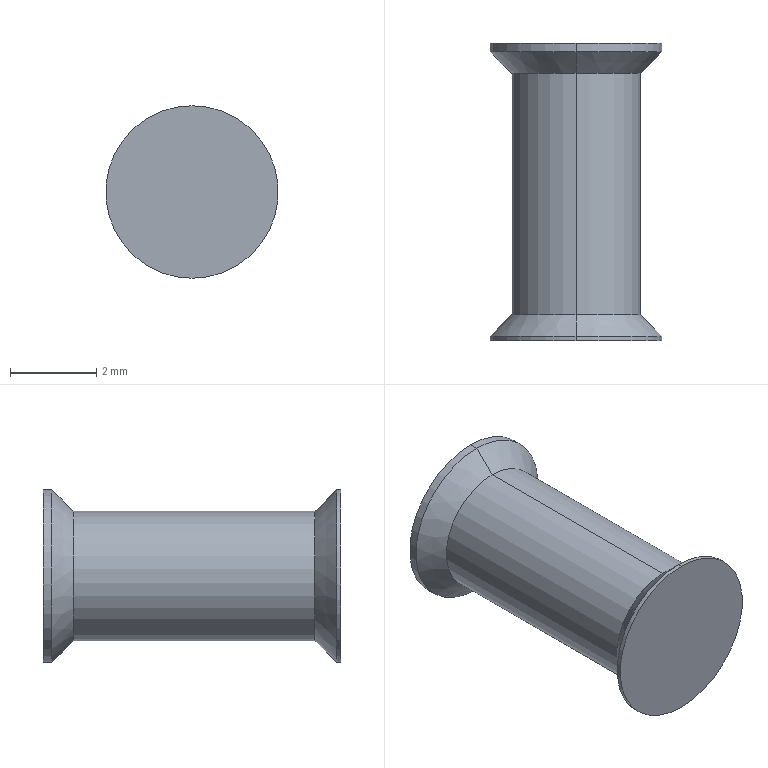Part | SolidWorks | features BaseBody 1 | 1 solid | 18 faces | box 4 x 6.9 x 4 mm | volume 46.627 mm3 | cylinder 8 | cone 6 | torus 2 | plane 2 | commonest cylinder face diameters 4 x4 2 x2 3 x2
STEP:
#1=CARTESIAN_POINT('',(0.,8.1,-1.3));
#2=VERTEX_POINT('',#1);
#3=CARTESIAN_POINT('',(0.,8.1,1.3));
#4=VERTEX_POINT('',#3);
#5=CARTESIAN_POINT('',(0.,8.1,0.));
#6=DIRECTION('',(0.,-1.,0.));
#7=DIRECTION('',(0.,0.,1.));
#8=AXIS2_PLACEMENT_3D('',#5,#6,#7);
#9=CIRCLE('',#8,1.3);
#10=EDGE_CURVE('',#2,#4,#9,.T.);
#11=ORIENTED_EDGE('',*,*,#10,.F.);
#12=CARTESIAN_POINT('',(0.,7.8,-1.));
#13=VERTEX_POINT('',#12);
#14=CARTESIAN_POINT('',(0.,7.8,-1.3));
#15=DIRECTION('',(1.,0.,0.));
#16=DIRECTION('',(0.,0.,-1.));
#17=AXIS2_PLACEMENT_3D('',#14,#15,#16);
#18=CIRCLE('',#17,0.3);
#19=EDGE_CURVE('',#2,#13,#18,.T.);
#20=ORIENTED_EDGE('',*,*,#19,.T.);
#21=CARTESIAN_POINT('',(0.,7.8,1.));
#22=VERTEX_POINT('',#21);
#23=CARTESIAN_POINT('',(0.,7.8,0.));
#24=DIRECTION('',(0.,1.,0.));
#25=DIRECTION('',(0.,0.,1.));
#26=AXIS2_PLACEMENT_3D('',#23,#24,#25);
#27=CIRCLE('',#26,1.);
#28=EDGE_CURVE('',#22,#13,#27,.T.);
#29=ORIENTED_EDGE('',*,*,#28,.F.);
#30=CARTESIAN_POINT('',(0.,7.8,1.3));
#31=DIRECTION('',(-1.,0.,0.));
#32=DIRECTION('',(0.,0.,1.));
#33=AXIS2_PLACEMENT_3D('',#30,#31,#32);
#34=CIRCLE('',#33,0.3);
#35=EDGE_CURVE('',#4,#22,#34,.T.);
#36=ORIENTED_EDGE('',*,*,#35,.F.);
#37=EDGE_LOOP('',(#11,#20,#29,#36));
#38=FACE_OUTER_BOUND('',#37,.T.);
#39=CARTESIAN_POINT('',(0.,7.8,0.));
#40=DIRECTION('',(0.,1.,0.));
#41=DIRECTION('',(0.,0.,1.));
#42=AXIS2_PLACEMENT_3D('',#39,#40,#41);
#43=TOROIDAL_SURFACE('',#42,1.3,0.3);
#44=ADVANCED_FACE('',(#38),#43,.T.);
#45=CARTESIAN_POINT('',(0.,7.8,0.));
#46=DIRECTION('',(0.,1.,0.));
#47=DIRECTION('',(0.,0.,1.));
#48=AXIS2_PLACEMENT_3D('',#45,#46,#47);
#49=CIRCLE('',#48,1.);
#50=EDGE_CURVE('',#13,#22,#49,.T.);
#51=ORIENTED_EDGE('',*,*,#50,.T.);
#52=CARTESIAN_POINT('',(0.,6.3,1.));
#53=VERTEX_POINT('',#52);
#54=CARTESIAN_POINT('',(0.,-2.993,1.));
#55=DIRECTION('',(0.,-1.,0.));
#56=VECTOR('',#55,1000.);
#57=LINE('',#54,#56);
#58=EDGE_CURVE('',#22,#53,#57,.T.);
#59=ORIENTED_EDGE('',*,*,#58,.T.);
#60=CARTESIAN_POINT('',(0.,6.3,-1.));
#61=VERTEX_POINT('',#60);
#62=CARTESIAN_POINT('',(0.,6.3,0.));
#63=DIRECTION('',(0.,-1.,0.));
#64=DIRECTION('',(0.,0.,-1.));
#65=AXIS2_PLACEMENT_3D('',#62,#63,#64);
#66=CIRCLE('',#65,1.);
#67=EDGE_CURVE('',#53,#61,#66,.T.);
#68=ORIENTED_EDGE('',*,*,#67,.T.);
#69=CARTESIAN_POINT('',(0.,-2.993,-1.));
#70=DIRECTION('',(0.,-1.,0.));
#71=VECTOR('',#70,1000.);
#72=LINE('',#69,#71);
#73=EDGE_CURVE('',#13,#61,#72,.T.);
#74=ORIENTED_EDGE('',*,*,#73,.F.);
#75=EDGE_LOOP('',(#51,#59,#68,#74));
#76=FACE_OUTER_BOUND('',#75,.T.);
#77=CARTESIAN_POINT('',(0.,-2.993,0.));
#78=DIRECTION('',(0.,-1.,0.));
#79=DIRECTION('',(0.,0.,-1.));
#80=AXIS2_PLACEMENT_3D('',#77,#78,#79);
#81=CYLINDRICAL_SURFACE('',#80,1.);
#82=ADVANCED_FACE('',(#76),#81,.F.);
#83=CARTESIAN_POINT('',(0.,5.699,0.));
#84=VERTEX_POINT('',#83);
#85=CARTESIAN_POINT('',(0.,6.3,1.));
#86=DIRECTION('',(0.,0.515,0.8572));
#87=VECTOR('',#86,1000.);
#88=LINE('',#85,#87);
#89=EDGE_CURVE('',#84,#53,#88,.T.);
#90=ORIENTED_EDGE('',*,*,#89,.F.);
#91=CARTESIAN_POINT('',(0.,6.3,-1.));
#92=DIRECTION('',(0.,0.515,-0.8572));
#93=VECTOR('',#92,1000.);
#94=LINE('',#91,#93);
#95=EDGE_CURVE('',#84,#61,#94,.T.);
#96=ORIENTED_EDGE('',*,*,#95,.T.);
#97=ORIENTED_EDGE('',*,*,#67,.F.);
#98=EDGE_LOOP('',(#90,#96,#97));
#99=FACE_OUTER_BOUND('',#98,.T.);
#100=CARTESIAN_POINT('',(0.,6.3,0.));
#101=DIRECTION('',(0.,1.,0.));
#102=DIRECTION('',(0.,0.,1.));
#103=AXIS2_PLACEMENT_3D('',#100,#101,#102);
#104=CONICAL_SURFACE('',#103,1.,1.03);
#105=ADVANCED_FACE('',(#99),#104,.F.);
#106=CARTESIAN_POINT('',(0.,7.4,1.5));
#107=VERTEX_POINT('',#106);
#108=CARTESIAN_POINT('',(0.,7.4,-1.5));
#109=VERTEX_POINT('',#108);
#110=CARTESIAN_POINT('',(0.,7.4,0.));
#111=DIRECTION('',(0.,1.,0.));
#112=DIRECTION('',(0.,0.,-1.));
#113=AXIS2_PLACEMENT_3D('',#110,#111,#112);
#114=CIRCLE('',#113,1.5);
#115=EDGE_CURVE('',#107,#109,#114,.T.);
#116=ORIENTED_EDGE('',*,*,#115,.T.);
#117=CARTESIAN_POINT('',(0.,7.9,-2.));
#118=VERTEX_POINT('',#117);
#119=CARTESIAN_POINT('',(0.,7.4,-1.5));
#120=DIRECTION('',(0.,0.7071,-0.7071));
#121=VECTOR('',#120,1000.);
#122=LINE('',#119,#121);
#123=EDGE_CURVE('',#109,#118,#122,.T.);
#124=ORIENTED_EDGE('',*,*,#123,.T.);
#125=CARTESIAN_POINT('',(0.,7.9,2.));
#126=VERTEX_POINT('',#125);
#127=CARTESIAN_POINT('',(0.,7.9,0.));
#128=DIRECTION('',(0.,1.,0.));
#129=DIRECTION('',(0.,0.,-1.));
#130=AXIS2_PLACEMENT_3D('',#127,#128,#129);
#131=CIRCLE('',#130,2.);
#132=EDGE_CURVE('',#126,#118,#131,.T.);
#133=ORIENTED_EDGE('',*,*,#132,.F.);
#134=CARTESIAN_POINT('',(0.,7.4,1.5));
#135=DIRECTION('',(0.,0.7071,0.7071));
#136=VECTOR('',#135,1000.);
#137=LINE('',#134,#136);
#138=EDGE_CURVE('',#107,#126,#137,.T.);
#139=ORIENTED_EDGE('',*,*,#138,.F.);
#140=EDGE_LOOP('',(#116,#124,#133,#139));
#141=FACE_OUTER_BOUND('',#140,.T.);
#142=CARTESIAN_POINT('',(0.,7.4,0.));
#143=DIRECTION('',(0.,1.,0.));
#144=DIRECTION('',(0.,0.,1.));
#145=AXIS2_PLACEMENT_3D('',#142,#143,#144);
#146=CONICAL_SURFACE('',#145,1.5,0.7854);
#147=ADVANCED_FACE('',(#141),#146,.T.);
#148=ORIENTED_EDGE('',*,*,#115,.F.);
#149=CARTESIAN_POINT('',(0.,1.8,1.5));
#150=VERTEX_POINT('',#149);
#151=CARTESIAN_POINT('',(0.,-2.993,1.5));
#152=DIRECTION('',(0.,-1.,0.));
#153=VECTOR('',#152,1000.);
#154=LINE('',#151,#153);
#155=EDGE_CURVE('',#107,#150,#154,.T.);
#156=ORIENTED_EDGE('',*,*,#155,.T.);
#157=CARTESIAN_POINT('',(0.,1.8,-1.5));
#158=VERTEX_POINT('',#157);
#159=CARTESIAN_POINT('',(0.,1.8,0.));
#160=DIRECTION('',(0.,-1.,0.));
#161=DIRECTION('',(0.,0.,1.));
#162=AXIS2_PLACEMENT_3D('',#159,#160,#161);
#163=CIRCLE('',#162,1.5);
#164=EDGE_CURVE('',#158,#150,#163,.T.);
#165=ORIENTED_EDGE('',*,*,#164,.F.);
#166=CARTESIAN_POINT('',(0.,-2.993,-1.5));
#167=DIRECTION('',(0.,-1.,0.));
#168=VECTOR('',#167,1000.);
#169=LINE('',#166,#168);
#170=EDGE_CURVE('',#109,#158,#169,.T.);
#171=ORIENTED_EDGE('',*,*,#170,.F.);
#172=EDGE_LOOP('',(#148,#156,#165,#171));
#173=FACE_OUTER_BOUND('',#172,.T.);
#174=CARTESIAN_POINT('',(0.,-2.993,0.));
#175=DIRECTION('',(0.,-1.,0.));
#176=DIRECTION('',(0.,0.,-1.));
#177=AXIS2_PLACEMENT_3D('',#174,#175,#176);
#178=CYLINDRICAL_SURFACE('',#177,1.5);
#179=ADVANCED_FACE('',(#173),#178,.T.);
#180=ORIENTED_EDGE('',*,*,#164,.T.);
#181=CARTESIAN_POINT('',(0.,1.3,2.));
#182=VERTEX_POINT('',#181);
#183=CARTESIAN_POINT('',(0.,1.3,2.));
#184=DIRECTION('',(0.,-0.7071,0.7071));
#185=VECTOR('',#184,1000.);
#186=LINE('',#183,#185);
#187=EDGE_CURVE('',#150,#182,#186,.T.);
#188=ORIENTED_EDGE('',*,*,#187,.T.);
#189=CARTESIAN_POINT('',(0.,1.3,-2.));
#190=VERTEX_POINT('',#189);
#191=CARTESIAN_POINT('',(0.,1.3,0.));
#192=DIRECTION('',(0.,-1.,0.));
#193=DIRECTION('',(0.,0.,-1.));
#194=AXIS2_PLACEMENT_3D('',#191,#192,#193);
#195=CIRCLE('',#194,2.);
#196=EDGE_CURVE('',#190,#182,#195,.T.);
#197=ORIENTED_EDGE('',*,*,#196,.F.);
#198=CARTESIAN_POINT('',(0.,1.3,-2.));
#199=DIRECTION('',(0.,-0.7071,-0.7071));
#200=VECTOR('',#199,1000.);
#201=LINE('',#198,#200);
#202=EDGE_CURVE('',#158,#190,#201,.T.);
#203=ORIENTED_EDGE('',*,*,#202,.F.);
#204=EDGE_LOOP('',(#180,#188,#197,#203));
#205=FACE_OUTER_BOUND('',#204,.T.);
#206=CARTESIAN_POINT('',(0.,1.3,0.));
#207=DIRECTION('',(0.,-1.,0.));
#208=DIRECTION('',(0.,0.,-1.));
#209=AXIS2_PLACEMENT_3D('',#206,#207,#208);
#210=CONICAL_SURFACE('',#209,2.,0.7854);
#211=ADVANCED_FACE('',(#205),#210,.T.);
#212=CARTESIAN_POINT('',(0.,1.2,-2.));
#213=VERTEX_POINT('',#212);
#214=CARTESIAN_POINT('',(0.,1.2,2.));
#215=VERTEX_POINT('',#214);
#216=CARTESIAN_POINT('',(0.,1.2,0.));
#217=DIRECTION('',(0.,-1.,0.));
#218=DIRECTION('',(0.,0.,-1.));
#219=AXIS2_PLACEMENT_3D('',#216,#217,#218);
#220=CIRCLE('',#219,2.);
#221=EDGE_CURVE('',#213,#215,#220,.T.);
#222=ORIENTED_EDGE('',*,*,#221,.F.);
#223=CARTESIAN_POINT('',(0.,1.2,-2.));
#224=DIRECTION('',(0.,1.,0.));
#225=VECTOR('',#224,1000.);
#226=LINE('',#223,#225);
#227=EDGE_CURVE('',#213,#190,#226,.T.);
#228=ORIENTED_EDGE('',*,*,#227,.T.);
#229=ORIENTED_EDGE('',*,*,#196,.T.);
#230=CARTESIAN_POINT('',(0.,1.2,2.));
#231=DIRECTION('',(0.,1.,0.));
#232=VECTOR('',#231,1000.);
#233=LINE('',#230,#232);
#234=EDGE_CURVE('',#215,#182,#233,.T.);
#235=ORIENTED_EDGE('',*,*,#234,.F.);
#236=EDGE_LOOP('',(#222,#228,#229,#235));
#237=FACE_OUTER_BOUND('',#236,.T.);
#238=CARTESIAN_POINT('',(0.,1.2,0.));
#239=DIRECTION('',(0.,1.,0.));
#240=DIRECTION('',(0.,0.,1.));
#241=AXIS2_PLACEMENT_3D('',#238,#239,#240);
#242=CYLINDRICAL_SURFACE('',#241,2.);
#243=ADVANCED_FACE('',(#237),#242,.T.);
#244=CARTESIAN_POINT('',(0.,8.1,-2.));
#245=VERTEX_POINT('',#244);
#246=CARTESIAN_POINT('',(0.,8.1,2.));
#247=VERTEX_POINT('',#246);
#248=CARTESIAN_POINT('',(0.,8.1,0.));
#249=DIRECTION('',(0.,-1.,0.));
#250=DIRECTION('',(0.,0.,1.));
#251=AXIS2_PLACEMENT_3D('',#248,#249,#250);
#252=CIRCLE('',#251,2.);
#253=EDGE_CURVE('',#245,#247,#252,.T.);
#254=ORIENTED_EDGE('',*,*,#253,.T.);
#255=CARTESIAN_POINT('',(0.,-2.993,2.));
#256=DIRECTION('',(0.,-1.,0.));
#257=VECTOR('',#256,1000.);
#258=LINE('',#255,#257);
#259=EDGE_CURVE('',#247,#126,#258,.T.);
#260=ORIENTED_EDGE('',*,*,#259,.T.);
#261=ORIENTED_EDGE('',*,*,#132,.T.);
#262=CARTESIAN_POINT('',(0.,-2.993,-2.));
#263=DIRECTION('',(0.,-1.,0.));
#264=VECTOR('',#263,1000.);
#265=LINE('',#262,#264);
#266=EDGE_CURVE('',#245,#118,#265,.T.);
#267=ORIENTED_EDGE('',*,*,#266,.F.);
#268=EDGE_LOOP('',(#254,#260,#261,#267));
#269=FACE_OUTER_BOUND('',#268,.T.);
#270=CARTESIAN_POINT('',(0.,-2.993,0.));
#271=DIRECTION('',(0.,-1.,0.));
#272=DIRECTION('',(0.,0.,-1.));
#273=AXIS2_PLACEMENT_3D('',#270,#271,#272);
#274=CYLINDRICAL_SURFACE('',#273,2.);
#275=ADVANCED_FACE('',(#269),#274,.T.);
#276=ORIENTED_EDGE('',*,*,#259,.F.);
#277=CARTESIAN_POINT('',(0.,8.1,0.));
#278=DIRECTION('',(0.,-1.,0.));
#279=DIRECTION('',(0.,0.,1.));
#280=AXIS2_PLACEMENT_3D('',#277,#278,#279);
#281=CIRCLE('',#280,2.);
#282=EDGE_CURVE('',#247,#245,#281,.T.);
#283=ORIENTED_EDGE('',*,*,#282,.T.);
#284=ORIENTED_EDGE('',*,*,#266,.T.);
#285=CARTESIAN_POINT('',(0.,7.9,0.));
#286=DIRECTION('',(0.,1.,0.));
#287=DIRECTION('',(0.,0.,-1.));
#288=AXIS2_PLACEMENT_3D('',#285,#286,#287);
#289=CIRCLE('',#288,2.);
#290=EDGE_CURVE('',#118,#126,#289,.T.);
#291=ORIENTED_EDGE('',*,*,#290,.T.);
#292=EDGE_LOOP('',(#276,#283,#284,#291));
#293=FACE_OUTER_BOUND('',#292,.T.);
#294=CARTESIAN_POINT('',(0.,-2.993,0.));
#295=DIRECTION('',(0.,-1.,0.));
#296=DIRECTION('',(0.,0.,-1.));
#297=AXIS2_PLACEMENT_3D('',#294,#295,#296);
#298=CYLINDRICAL_SURFACE('',#297,2.);
#299=ADVANCED_FACE('',(#293),#298,.T.);
#300=CARTESIAN_POINT('',(0.,1.2,0.));
#301=DIRECTION('',(0.,-1.,0.));
#302=DIRECTION('',(0.,0.,-1.));
#303=AXIS2_PLACEMENT_3D('',#300,#301,#302);
#304=CIRCLE('',#303,2.);
#305=EDGE_CURVE('',#215,#213,#304,.T.);
#306=ORIENTED_EDGE('',*,*,#305,.T.);
#307=ORIENTED_EDGE('',*,*,#221,.T.);
#308=EDGE_LOOP('',(#306,#307));
#309=FACE_OUTER_BOUND('',#308,.T.);
#310=CARTESIAN_POINT('',(0.,1.2,0.));
#311=DIRECTION('',(0.,-1.,0.));
#312=DIRECTION('',(0.,0.,-1.));
#313=AXIS2_PLACEMENT_3D('',#310,#311,#312);
#314=PLANE('',#313);
#315=ADVANCED_FACE('',(#309),#314,.T.);
#316=ORIENTED_EDGE('',*,*,#227,.F.);
#317=ORIENTED_EDGE('',*,*,#305,.F.);
#318=ORIENTED_EDGE('',*,*,#234,.T.);
#319=CARTESIAN_POINT('',(0.,1.3,0.));
#320=DIRECTION('',(0.,-1.,0.));
#321=DIRECTION('',(0.,0.,-1.));
#322=AXIS2_PLACEMENT_3D('',#319,#320,#321);
#323=CIRCLE('',#322,2.);
#324=EDGE_CURVE('',#182,#190,#323,.T.);
#325=ORIENTED_EDGE('',*,*,#324,.T.);
#326=EDGE_LOOP('',(#316,#317,#318,#325));
#327=FACE_OUTER_BOUND('',#326,.T.);
#328=CARTESIAN_POINT('',(0.,1.2,0.));
#329=DIRECTION('',(0.,1.,0.));
#330=DIRECTION('',(0.,0.,1.));
#331=AXIS2_PLACEMENT_3D('',#328,#329,#330);
#332=CYLINDRICAL_SURFACE('',#331,2.);
#333=ADVANCED_FACE('',(#327),#332,.T.);
#334=ORIENTED_EDGE('',*,*,#187,.F.);
#335=CARTESIAN_POINT('',(0.,1.8,0.));
#336=DIRECTION('',(0.,-1.,0.));
#337=DIRECTION('',(0.,0.,1.));
#338=AXIS2_PLACEMENT_3D('',#335,#336,#337);
#339=CIRCLE('',#338,1.5);
#340=EDGE_CURVE('',#150,#158,#339,.T.);
#341=ORIENTED_EDGE('',*,*,#340,.T.);
#342=ORIENTED_EDGE('',*,*,#202,.T.);
#343=ORIENTED_EDGE('',*,*,#324,.F.);
#344=EDGE_LOOP('',(#334,#341,#342,#343));
#345=FACE_OUTER_BOUND('',#344,.T.);
#346=CARTESIAN_POINT('',(0.,1.3,0.));
#347=DIRECTION('',(0.,-1.,0.));
#348=DIRECTION('',(0.,0.,-1.));
#349=AXIS2_PLACEMENT_3D('',#346,#347,#348);
#350=CONICAL_SURFACE('',#349,2.,0.7854);
#351=ADVANCED_FACE('',(#345),#350,.T.);
#352=ORIENTED_EDGE('',*,*,#155,.F.);
#353=CARTESIAN_POINT('',(0.,7.4,0.));
#354=DIRECTION('',(0.,1.,0.));
#355=DIRECTION('',(0.,0.,-1.));
#356=AXIS2_PLACEMENT_3D('',#353,#354,#355);
#357=CIRCLE('',#356,1.5);
#358=EDGE_CURVE('',#109,#107,#357,.T.);
#359=ORIENTED_EDGE('',*,*,#358,.F.);
#360=ORIENTED_EDGE('',*,*,#170,.T.);
#361=ORIENTED_EDGE('',*,*,#340,.F.);
#362=EDGE_LOOP('',(#352,#359,#360,#361));
#363=FACE_OUTER_BOUND('',#362,.T.);
#364=CARTESIAN_POINT('',(0.,-2.993,0.));
#365=DIRECTION('',(0.,-1.,0.));
#366=DIRECTION('',(0.,0.,-1.));
#367=AXIS2_PLACEMENT_3D('',#364,#365,#366);
#368=CYLINDRICAL_SURFACE('',#367,1.5);
#369=ADVANCED_FACE('',(#363),#368,.T.);
#370=ORIENTED_EDGE('',*,*,#123,.F.);
#371=ORIENTED_EDGE('',*,*,#358,.T.);
#372=ORIENTED_EDGE('',*,*,#138,.T.);
#373=ORIENTED_EDGE('',*,*,#290,.F.);
#374=EDGE_LOOP('',(#370,#371,#372,#373));
#375=FACE_OUTER_BOUND('',#374,.T.);
#376=CARTESIAN_POINT('',(0.,7.4,0.));
#377=DIRECTION('',(0.,1.,0.));
#378=DIRECTION('',(0.,0.,1.));
#379=AXIS2_PLACEMENT_3D('',#376,#377,#378);
#380=CONICAL_SURFACE('',#379,1.5,0.7854);
#381=ADVANCED_FACE('',(#375),#380,.T.);
#382=CARTESIAN_POINT('',(0.,8.1,0.));
#383=DIRECTION('',(0.,-1.,0.));
#384=DIRECTION('',(0.,0.,1.));
#385=AXIS2_PLACEMENT_3D('',#382,#383,#384);
#386=CIRCLE('',#385,1.3);
#387=EDGE_CURVE('',#4,#2,#386,.T.);
#388=ORIENTED_EDGE('',*,*,#387,.T.);
#389=ORIENTED_EDGE('',*,*,#10,.T.);
#390=EDGE_LOOP('',(#388,#389));
#391=FACE_BOUND('',#390,.T.);
#392=ORIENTED_EDGE('',*,*,#253,.F.);
#393=ORIENTED_EDGE('',*,*,#282,.F.);
#394=EDGE_LOOP('',(#392,#393));
#395=FACE_OUTER_BOUND('',#394,.T.);
#396=CARTESIAN_POINT('',(0.,8.1,0.));
#397=DIRECTION('',(0.,1.,0.));
#398=DIRECTION('',(0.,0.,1.));
#399=AXIS2_PLACEMENT_3D('',#396,#397,#398);
#400=PLANE('',#399);
#401=ADVANCED_FACE('',(#391,#395),#400,.T.);
#402=ORIENTED_EDGE('',*,*,#95,.F.);
#403=ORIENTED_EDGE('',*,*,#89,.T.);
#404=CARTESIAN_POINT('',(0.,6.3,0.));
#405=DIRECTION('',(0.,-1.,0.));
#406=DIRECTION('',(0.,0.,-1.));
#407=AXIS2_PLACEMENT_3D('',#404,#405,#406);
#408=CIRCLE('',#407,1.);
#409=EDGE_CURVE('',#61,#53,#408,.T.);
#410=ORIENTED_EDGE('',*,*,#409,.F.);
#411=EDGE_LOOP('',(#402,#403,#410));
#412=FACE_OUTER_BOUND('',#411,.T.);
#413=CARTESIAN_POINT('',(0.,6.3,0.));
#414=DIRECTION('',(0.,1.,0.));
#415=DIRECTION('',(0.,0.,1.));
#416=AXIS2_PLACEMENT_3D('',#413,#414,#415);
#417=CONICAL_SURFACE('',#416,1.,1.03);
#418=ADVANCED_FACE('',(#412),#417,.F.);
#419=ORIENTED_EDGE('',*,*,#58,.F.);
#420=ORIENTED_EDGE('',*,*,#28,.T.);
#421=ORIENTED_EDGE('',*,*,#73,.T.);
#422=ORIENTED_EDGE('',*,*,#409,.T.);
#423=EDGE_LOOP('',(#419,#420,#421,#422));
#424=FACE_OUTER_BOUND('',#423,.T.);
#425=CARTESIAN_POINT('',(0.,-2.993,0.));
#426=DIRECTION('',(0.,-1.,0.));
#427=DIRECTION('',(0.,0.,-1.));
#428=AXIS2_PLACEMENT_3D('',#425,#426,#427);
#429=CYLINDRICAL_SURFACE('',#428,1.);
#430=ADVANCED_FACE('',(#424),#429,.F.);
#431=ORIENTED_EDGE('',*,*,#19,.F.);
#432=ORIENTED_EDGE('',*,*,#387,.F.);
#433=ORIENTED_EDGE('',*,*,#35,.T.);
#434=ORIENTED_EDGE('',*,*,#50,.F.);
#435=EDGE_LOOP('',(#431,#432,#433,#434));
#436=FACE_OUTER_BOUND('',#435,.T.);
#437=CARTESIAN_POINT('',(0.,7.8,0.));
#438=DIRECTION('',(0.,1.,0.));
#439=DIRECTION('',(0.,0.,1.));
#440=AXIS2_PLACEMENT_3D('',#437,#438,#439);
#441=TOROIDAL_SURFACE('',#440,1.3,0.3);
#442=ADVANCED_FACE('',(#436),#441,.T.);
#443=CLOSED_SHELL('',(#44,#82,#105,#147,#179,#211,#243,#275,#299,#315,#333,#351,#369,#381,#401,#418,#430,#442));
#444=MANIFOLD_SOLID_BREP('',#443);
#445=CARTESIAN_POINT('',(0.,0.,0.));
#446=DIRECTION('',(0.,0.,1.));
#447=DIRECTION('',(1.,0.,0.));
#448=AXIS2_PLACEMENT_3D('',#445,#446,#447);
#449=(LENGTH_UNIT()NAMED_UNIT(*)SI_UNIT(.MILLI.,.METRE.));
#450=UNCERTAINTY_MEASURE_WITH_UNIT(LENGTH_MEASURE(0.00001),#449,'','');
#451=(NAMED_UNIT(*)PLANE_ANGLE_UNIT()SI_UNIT($,.RADIAN.));
#452=(NAMED_UNIT(*)SI_UNIT($,.STERADIAN.)SOLID_ANGLE_UNIT());
#453=(GEOMETRIC_REPRESENTATION_CONTEXT(3)GLOBAL_UNCERTAINTY_ASSIGNED_CONTEXT((#450))GLOBAL_UNIT_ASSIGNED_CONTEXT((#449,#451,#452))REPRESENTATION_CONTEXT('',''));
#454=ADVANCED_BREP_SHAPE_REPRESENTATION('',(#444,#448),#453);